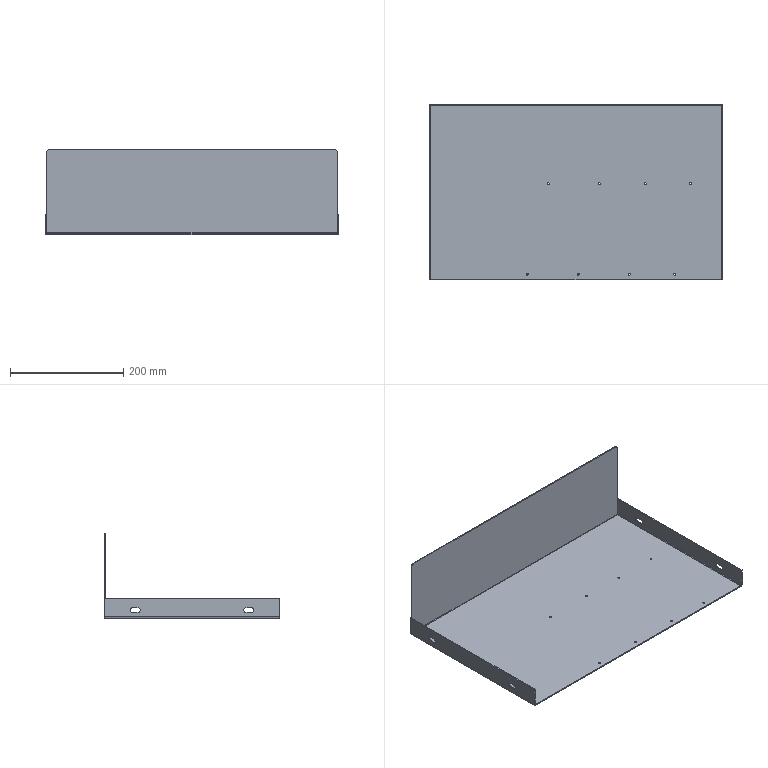Part | STEP file | 工作台二电气安装Plate | 1 solid | 66 faces | box 518 x 310 x 150 mm | volume 510899 mm3 | plane 34 | cylinder 32 | commonest cylinder face diameters 3.3 x16 8 x8 1.473 x3 5.473 x3 10 x2